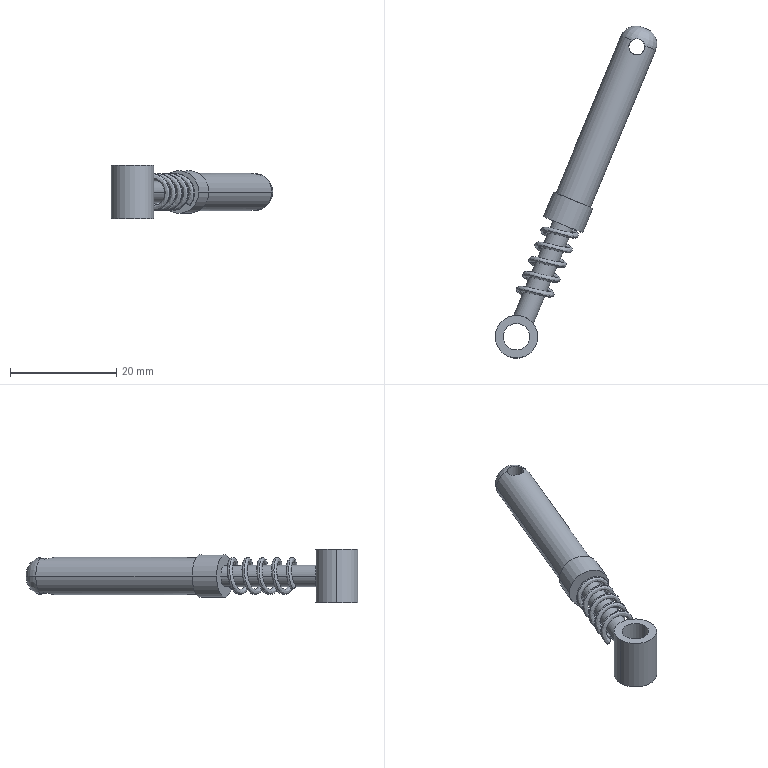Part | SolidWorks | features ICE 4, 3DProfileFeature 2, Extrusion 1, Fillet 1, Helix 1, Sweep 1 | 2 solids | 23 faces | box 30.391 x 62.421 x 10 mm | volume 2131 mm3 | cylinder 12 | plane 7 | torus 2 | spline 2 | commonest cylinder face diameters 8 x4 3 x2 4 x2 5 x2 7 x2